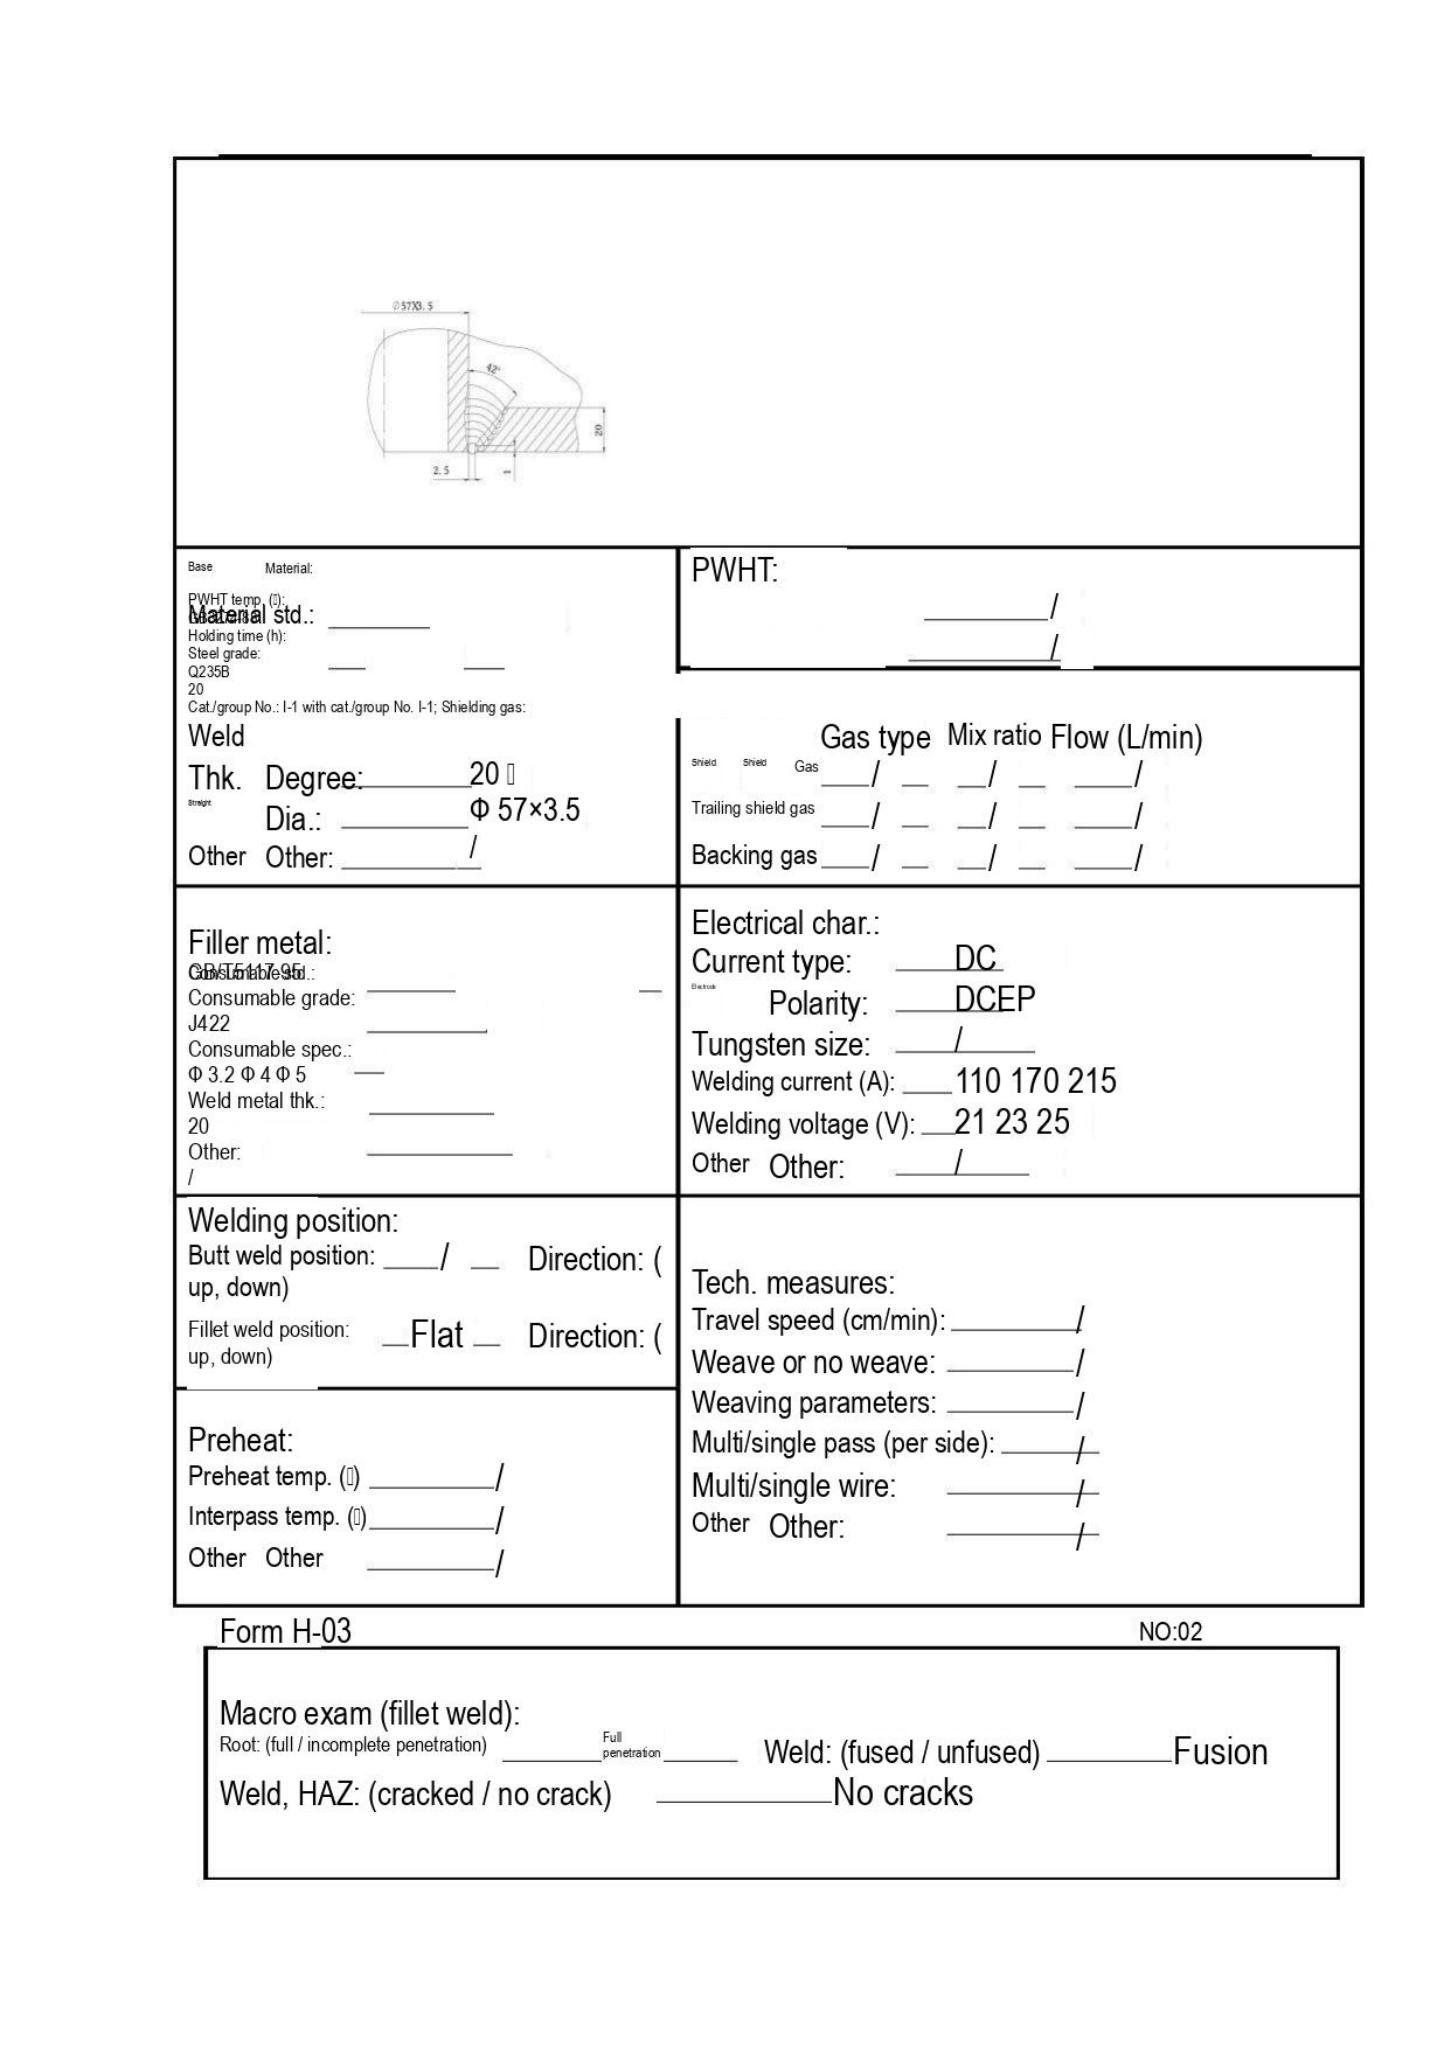Φ57X3.5

42°

20

2.5

1

Base Material:

PWHT temp. ():

Material std.:

Holding time (h):

Steel grade:

Q235B

20

Cat./group No.: I-1 with cat./group No. I-1; Shielding gas:

PWHT:

/

/

Weld

Thk. Degree: 20

Straight Dia.: Φ 57×3.5

Other Other: /

| | Gas type | Mix ratio | Flow (L/min) |
|---|---|---|---|
| Shield Shield Gas | / | / | / |
| Trailing shield gas | / | / | / |
| Backing gas | / | / | / |

Filler metal:

Consumable std.:

GB/T5117-95

Consumable grade:

J422

Consumable spec.:

Φ 3.2 Φ 4 Φ 5

Weld metal thk.:

20

Other:

/

Electrical char.:

Current type: DC

Electrode Polarity: DCEP

Tungsten size: /

Welding current (A): 110 170 215

Welding voltage (V): 21 23 25

Other Other: /

Welding position:

Butt weld position: / Direction: ( up, down)

Fillet weld position: Flat Direction: ( up, down)

Tech. measures:

Travel speed (cm/min): /

Weave or no weave: /

Weaving parameters: /

Multi/single pass (per side): /

Multi/single wire: /

Other Other: /

Preheat:

Preheat temp. () /

Interpass temp. () /

Other Other /

Form H-03

NO:02

Macro exam (fillet weld):

Root: (full / incomplete penetration) Full penetration

Weld: (fused / unfused) Fusion

Weld, HAZ: (cracked / no crack) No cracks
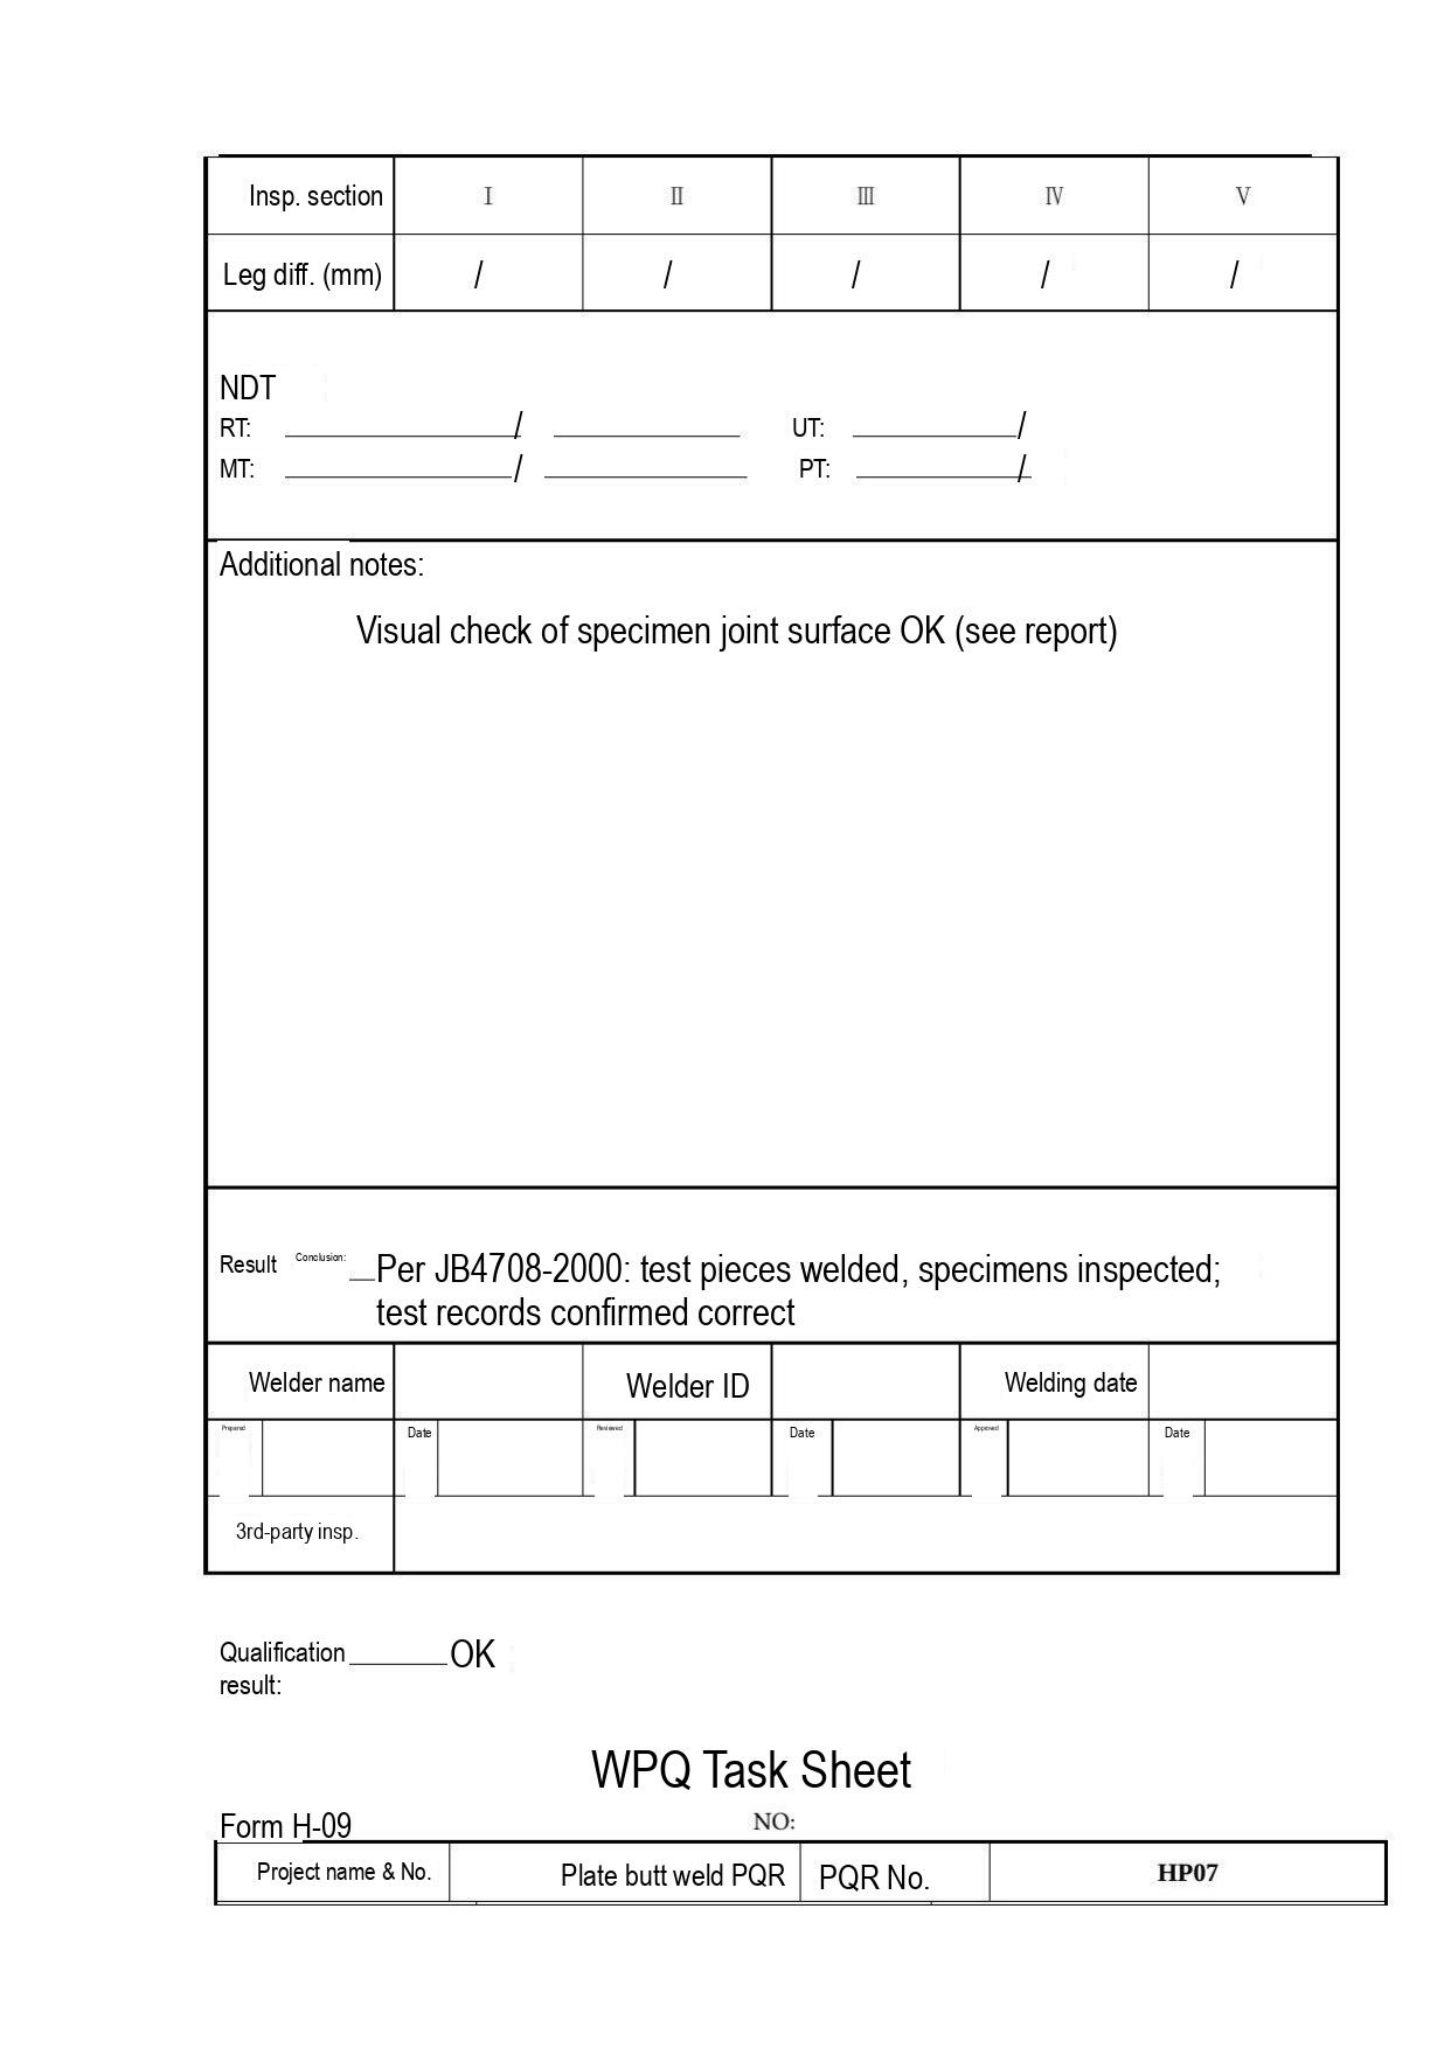| Insp. section | I | II | III | IV | V |
|---|---|---|---|---|---|
| Leg diff. (mm) | / | / | / | / | / |

NDT
RT: / UT: /
MT: / PT: /

Additional notes:

Visual check of specimen joint surface OK (see report)

Result Conclusion: Per JB4708-2000: test pieces welded, specimens inspected; test records confirmed correct

| Welder name | | Welder ID | | Welding date | |
|---|---|---|---|---|---|
| Prepared | Date | Reviewed | Date | Approved | Date |
| 3rd-party insp. | | | | | |

Qualification result: OK

WPQ Task Sheet

Form H-09 NO:

| Project name & No. | Plate butt weld PQR | PQR No. | HP07 |
|---|---|---|---|
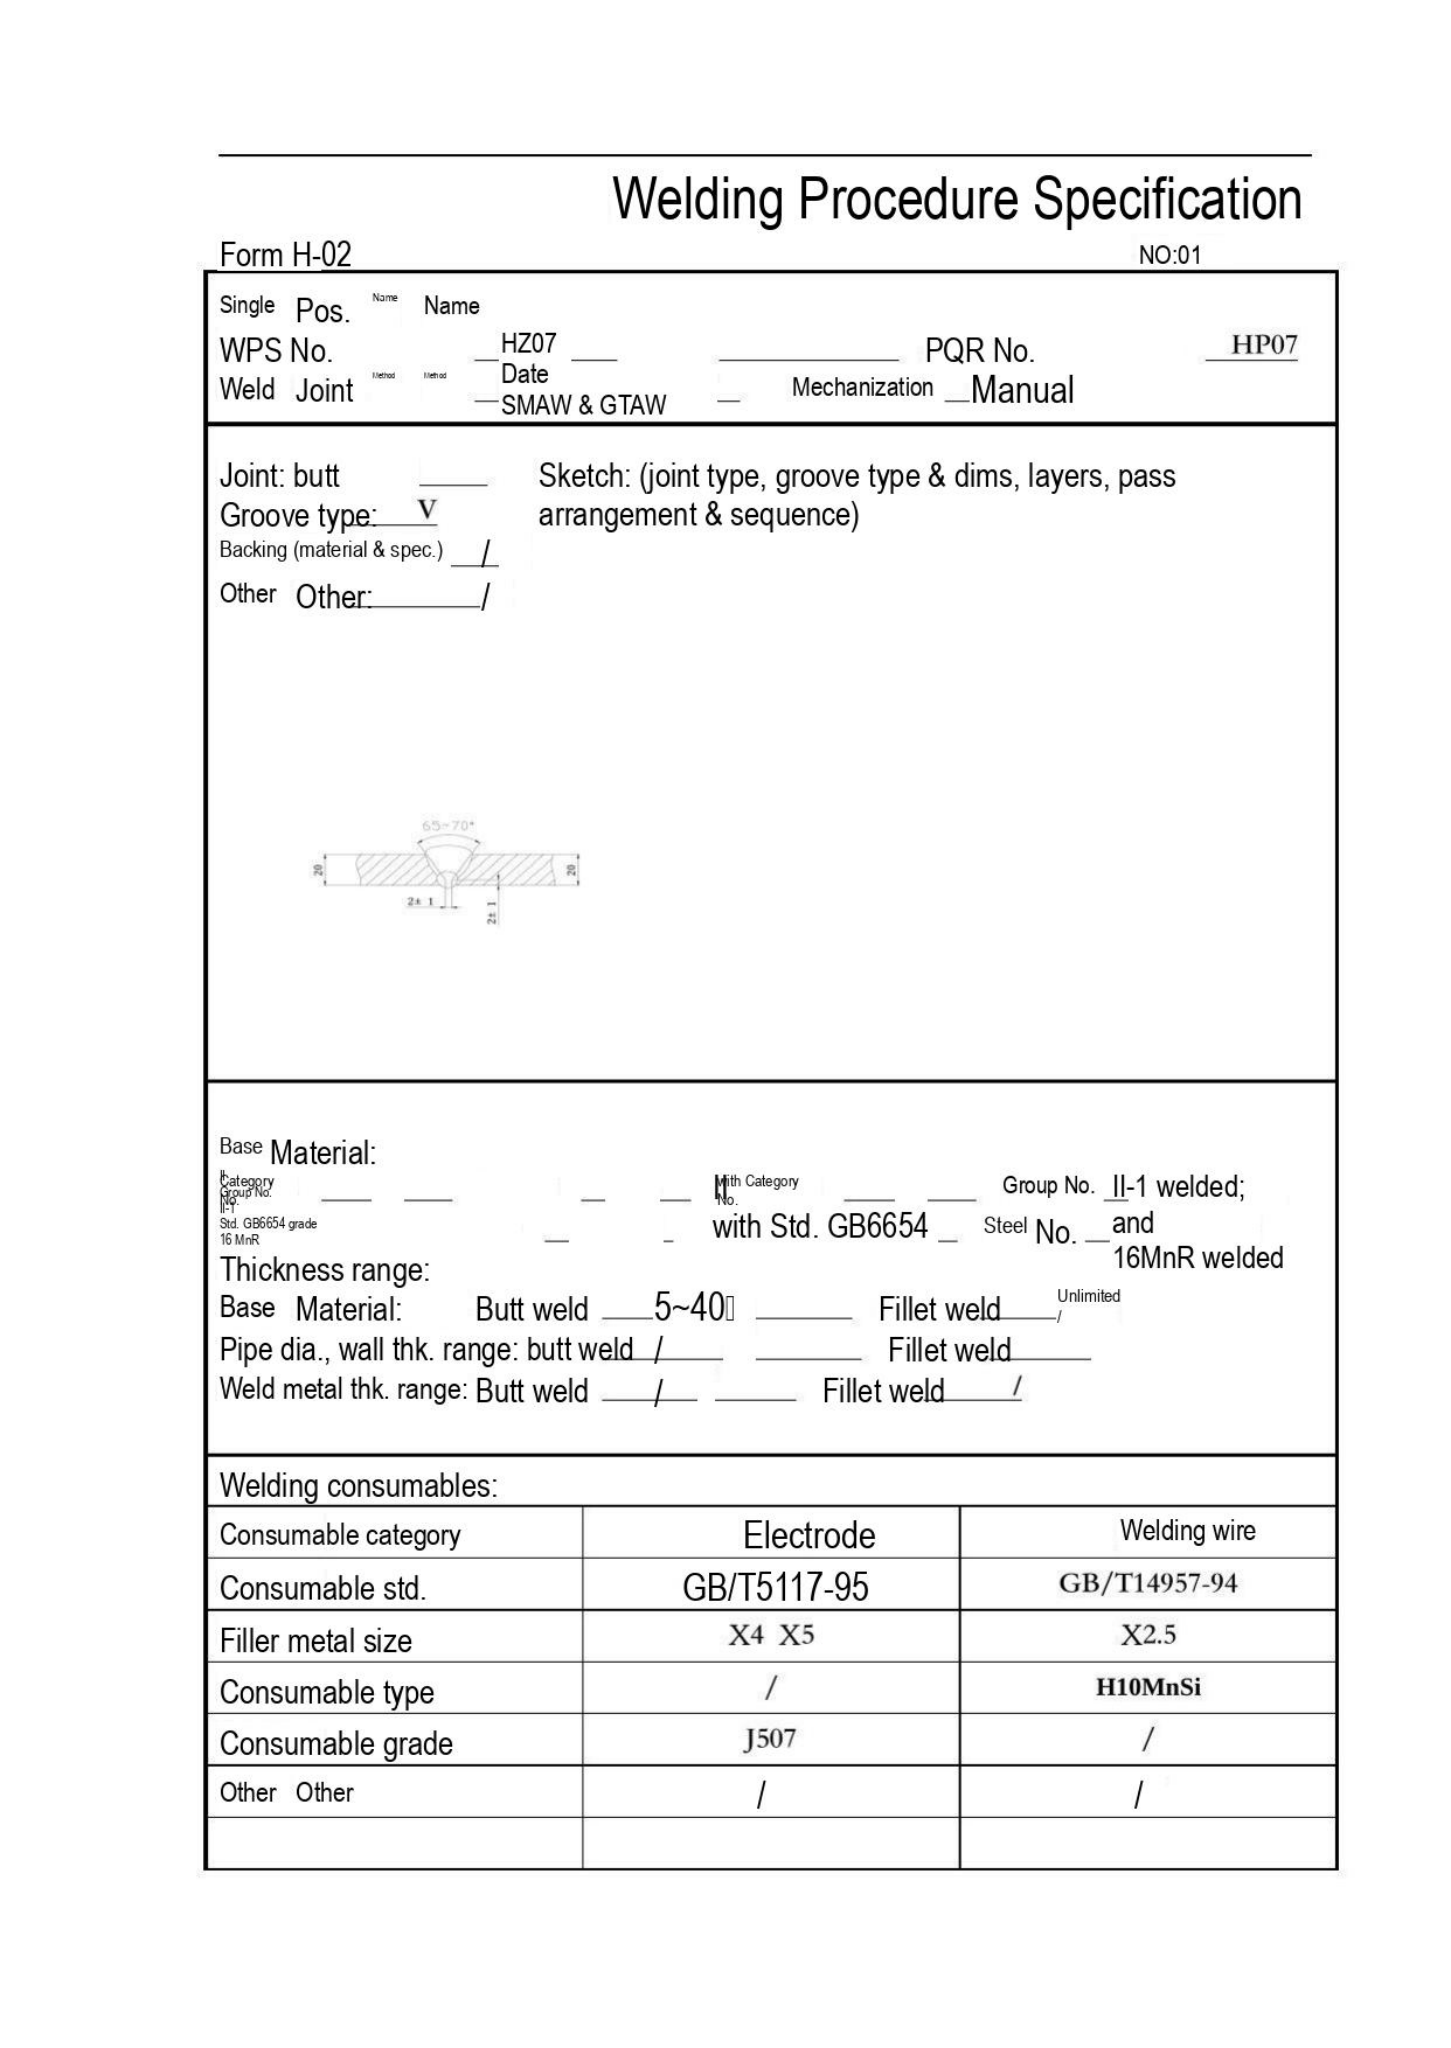Welding Procedure Specification

Form H-02 NO:01

Single Pos. Name Name
WPS No. HZ07 PQR No. HP07
Weld Joint Method Method Date SMAW & GTAW Mechanization Manual

Joint: butt
Groove type: V
Backing (material & spec.) /
Other Other: /

Sketch: (joint type, groove type & dims, layers, pass arrangement & sequence)

65~70°
20
20
2± 1
2± 1

Base Material:
II Category Group No. II-1
Std. GB6654 grade 16 MnR
II with Category No.
Group No. II-1 welded;
with Std. GB6654 Steel No. and 16MnR welded
Thickness range:
Base Material: Butt weld 5~40 Fillet weld Unlimited /
Pipe dia., wall thk. range: butt weld / Fillet weld
Weld metal thk. range: Butt weld / Fillet weld /

Welding consumables:

| Consumable category | Electrode | Welding wire |
|---|---|---|
| Consumable std. | GB/T5117-95 | GB/T14957-94 |
| Filler metal size | X4 X5 | X2.5 |
| Consumable type | / | H10MnSi |
| Consumable grade | J507 | / |
| Other Other | / | / |
| | | |
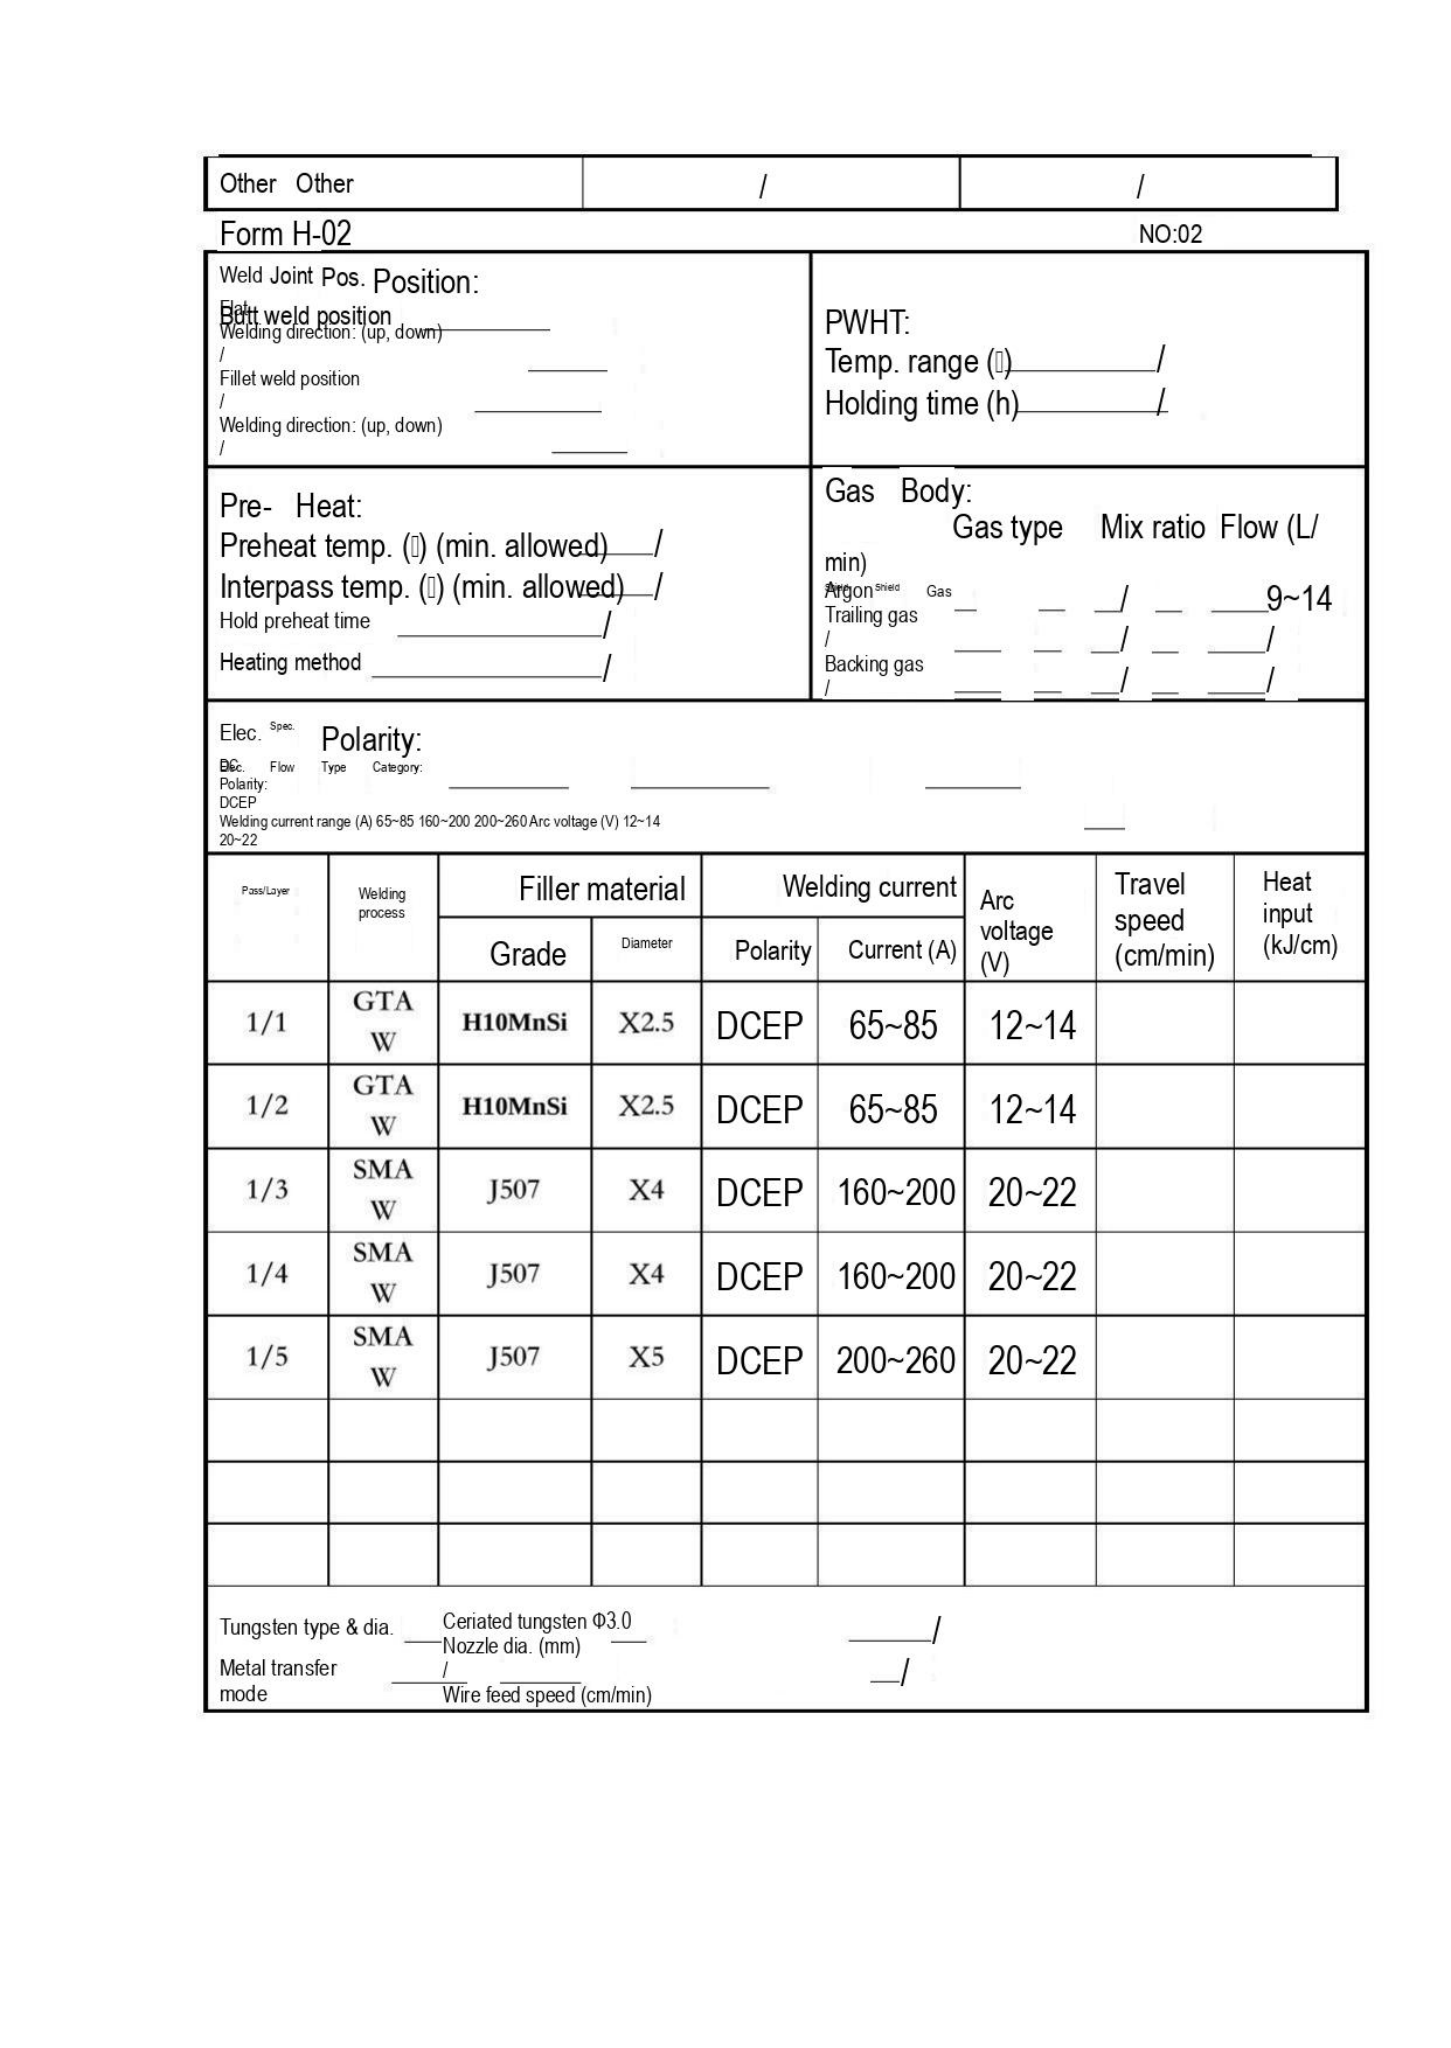| Other Other | / | / |
|---|---|---|

Form H-02

NO:02

Weld Joint Pos. Position:
Flat
Butt weld position
Welding direction: (up, down)
/
Fillet weld position
/
Welding direction: (up, down)
/

PWHT:
Temp. range (℃) /
Holding time (h) /

Pre- Heat:
Preheat temp. (℃) (min. allowed) /
Interpass temp. (℃) (min. allowed) /
Hold preheat time /
Heating method /

Gas Body:
Gas type Mix ratio Flow (L/min)
Shield Gas Argon / 9~14
Trailing gas / / /
Backing gas / / /

Elec. Spec. Polarity:
Elec. Flow Type Category: DC
Polarity:
DCEP
Welding current range (A) 65~85 160~200 200~260 Arc voltage (V) 12~14 20~22

| Pass/Layer | Welding process | Filler material: Grade | Filler material: Diameter | Welding current: Polarity | Welding current: Current (A) | Arc voltage (V) | Travel speed (cm/min) | Heat input (kJ/cm) |
|---|---|---|---|---|---|---|---|---|
| 1/1 | GTAW | H10MnSi | X2.5 | DCEP | 65~85 | 12~14 | | |
| 1/2 | GTAW | H10MnSi | X2.5 | DCEP | 65~85 | 12~14 | | |
| 1/3 | SMAW | J507 | X4 | DCEP | 160~200 | 20~22 | | |
| 1/4 | SMAW | J507 | X4 | DCEP | 160~200 | 20~22 | | |
| 1/5 | SMAW | J507 | X5 | DCEP | 200~260 | 20~22 | | |
| | | | | | | | | |
| | | | | | | | | |
| | | | | | | | | |

Tungsten type & dia. Ceriated tungsten Φ3.0
Nozzle dia. (mm) /
Metal transfer mode /
Wire feed speed (cm/min) /
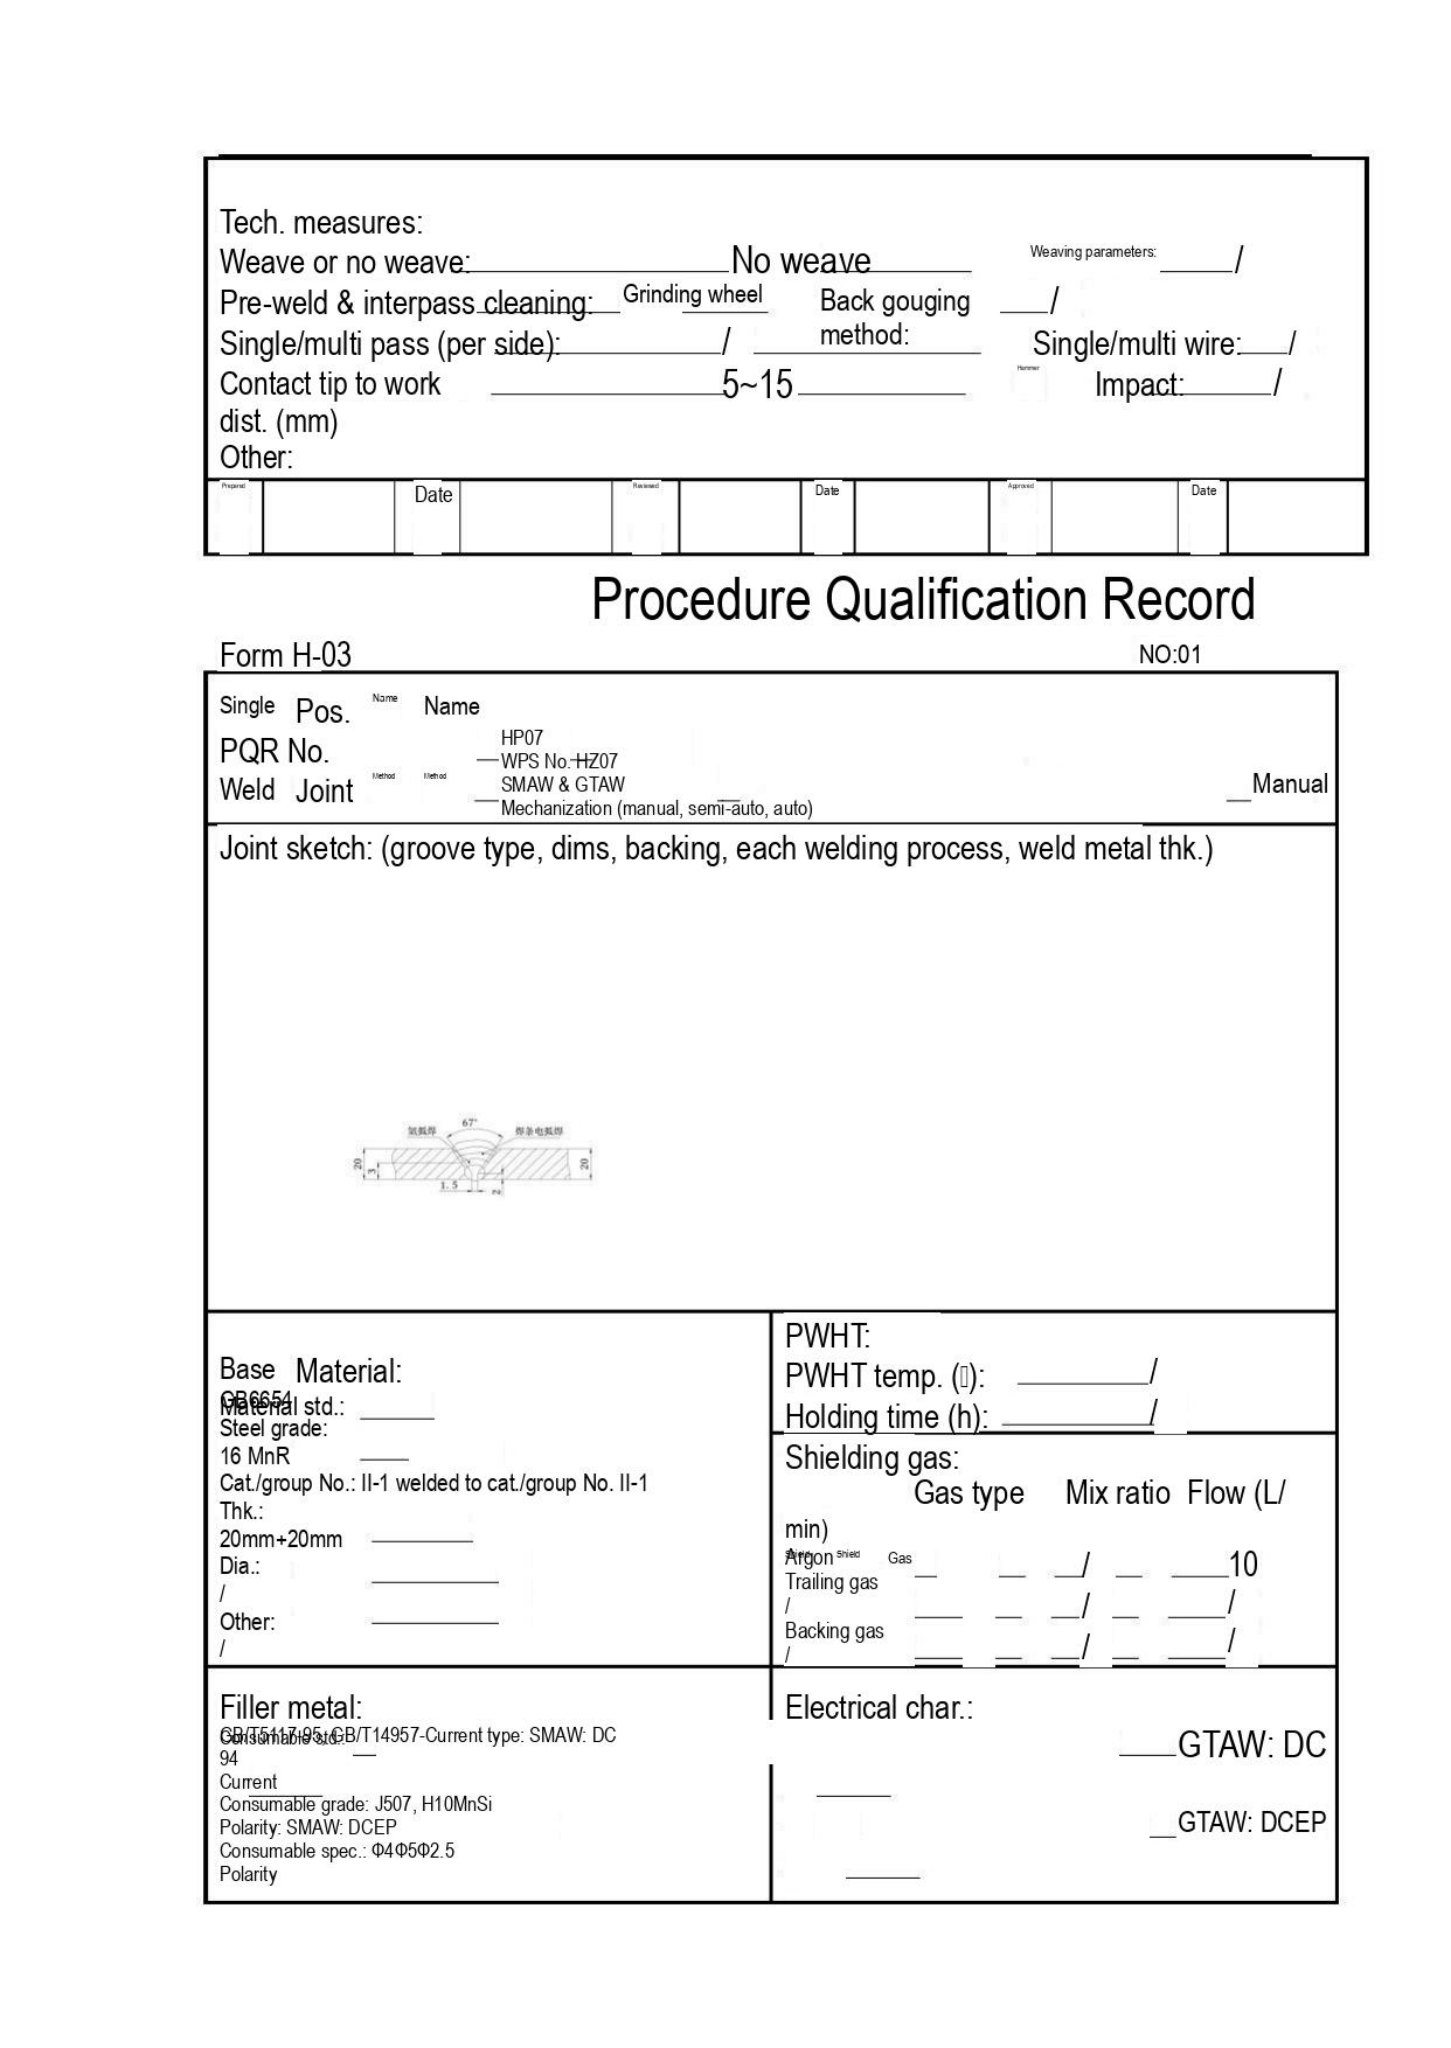Tech. measures:
Weave or no weave: No weave
Weaving parameters: /
Pre-weld & interpass cleaning: Grinding wheel
Back gouging method: /
Single/multi pass (per side): /
Single/multi wire: /
Contact tip to work dist. (mm) 5~15
Hammer
Impact: /
Other:

| Prepared | | Date | | Reviewed | | Date | | Approved | | Date | |
|---|---|---|---|---|---|---|---|---|---|---|---|

Procedure Qualification Record

Form H-03
NO:01

Single Pos. Name Name
PQR No. HP07
WPS No. HZ07
Weld Joint Method Method SMAW & GTAW
Mechanization (manual, semi-auto, auto) Manual

Joint sketch: (groove type, dims, backing, each welding process, weld metal thk.)

氩弧焊 67° 焊条电弧焊
20 3 20
1.5 P4

Base Material:
Material std.: GB6654
Steel grade: 16 MnR
Cat./group No.: II-1 welded to cat./group No. II-1
Thk.: 20mm+20mm
Dia.: /
Other: /

PWHT:
PWHT temp. (): /
Holding time (h): /

Shielding gas:
Gas type Mix ratio Flow (L/min)
Shield Gas Argon / 10
Trailing gas / /
Backing gas / /

Filler metal:
Consumable std.: GB/T5117-95, GB/T14957-94
Current type: SMAW: DC
Current
Consumable grade: J507, H10MnSi
Polarity: SMAW: DCEP
Consumable spec.: Φ4Φ5Φ2.5
Polarity

Electrical char.:
GTAW: DC
GTAW: DCEP
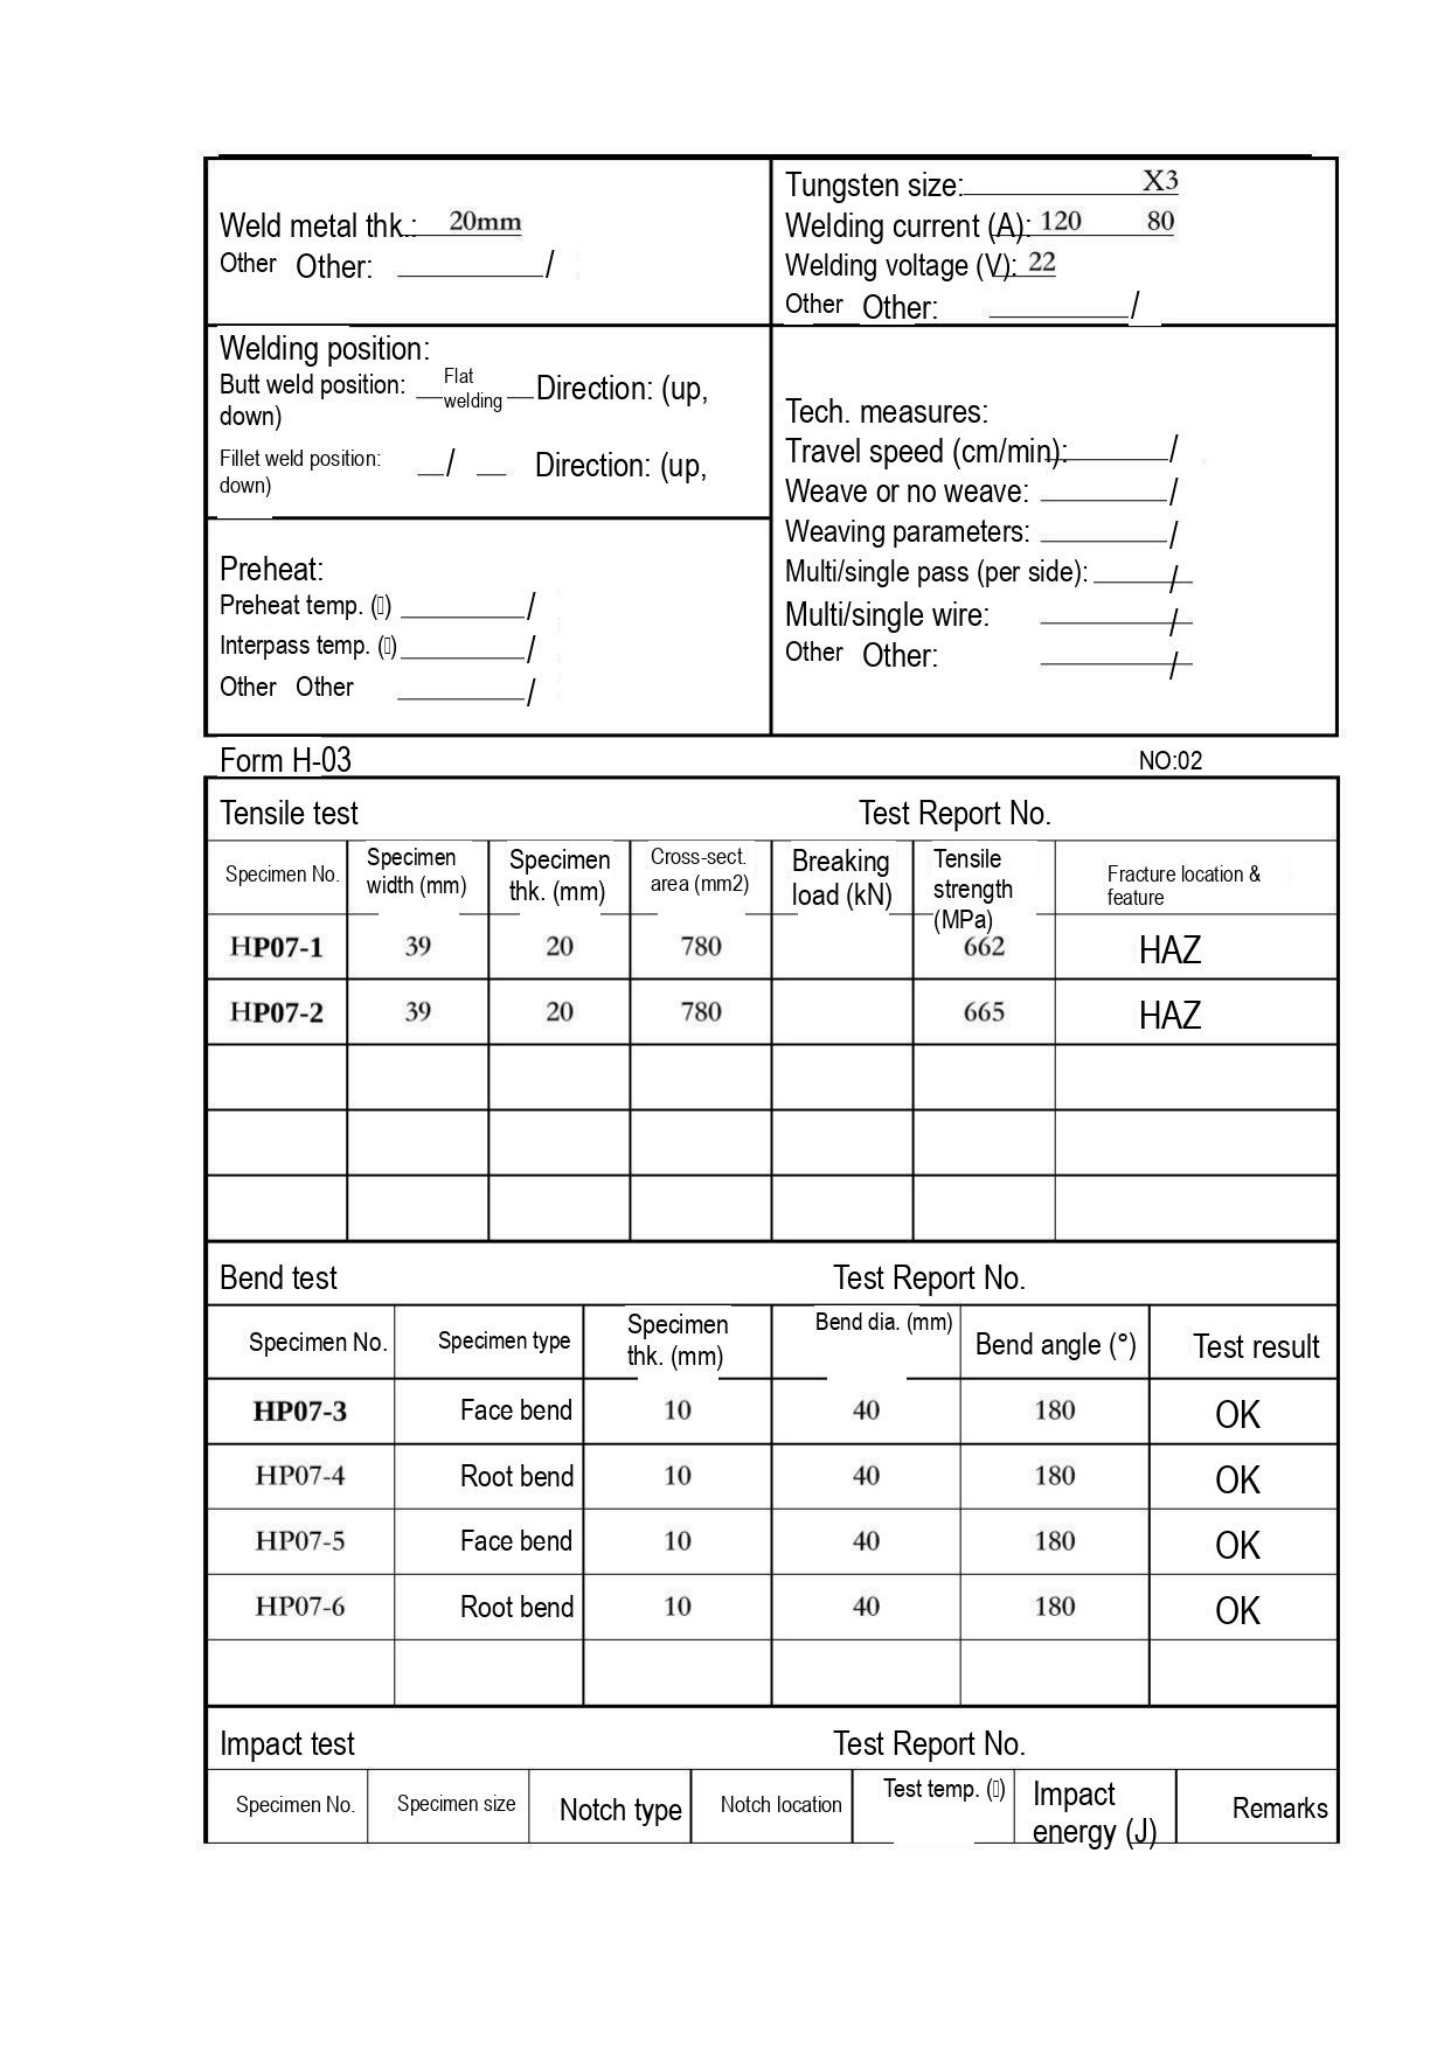| Weld metal thk.: 20mm<br>Other Other: / | Tungsten size: X3<br>Welding current (A): 120 80<br>Welding voltage (V): 22<br>Other Other: / |
|---|---|
| Welding position:<br>Butt weld position: Flat welding Direction: (up, down)<br>Fillet weld position: / Direction: (up, down) | Tech. measures:<br>Travel speed (cm/min): /<br>Weave or no weave: /<br>Weaving parameters: /<br>Multi/single pass (per side): /<br>Multi/single wire: /<br>Other Other: / |
| Preheat:<br>Preheat temp. ( ) /<br>Interpass temp. ( ) /<br>Other Other / | |

Form H-03 NO:02

Tensile test Test Report No.

| Specimen No. | Specimen width (mm) | Specimen thk. (mm) | Cross-sect. area (mm2) | Breaking load (kN) | Tensile strength (MPa) | Fracture location & feature |
|---|---|---|---|---|---|---|
| HP07-1 | 39 | 20 | 780 | | 662 | HAZ |
| HP07-2 | 39 | 20 | 780 | | 665 | HAZ |
| | | | | | | |
| | | | | | | |
| | | | | | | |

Bend test Test Report No.

| Specimen No. | Specimen type | Specimen thk. (mm) | Bend dia. (mm) | Bend angle (°) | Test result |
|---|---|---|---|---|---|
| HP07-3 | Face bend | 10 | 40 | 180 | OK |
| HP07-4 | Root bend | 10 | 40 | 180 | OK |
| HP07-5 | Face bend | 10 | 40 | 180 | OK |
| HP07-6 | Root bend | 10 | 40 | 180 | OK |
| | | | | | |

Impact test Test Report No.

| Specimen No. | Specimen size | Notch type | Notch location | Test temp. ( ) | Impact energy (J) | Remarks |
|---|---|---|---|---|---|---|
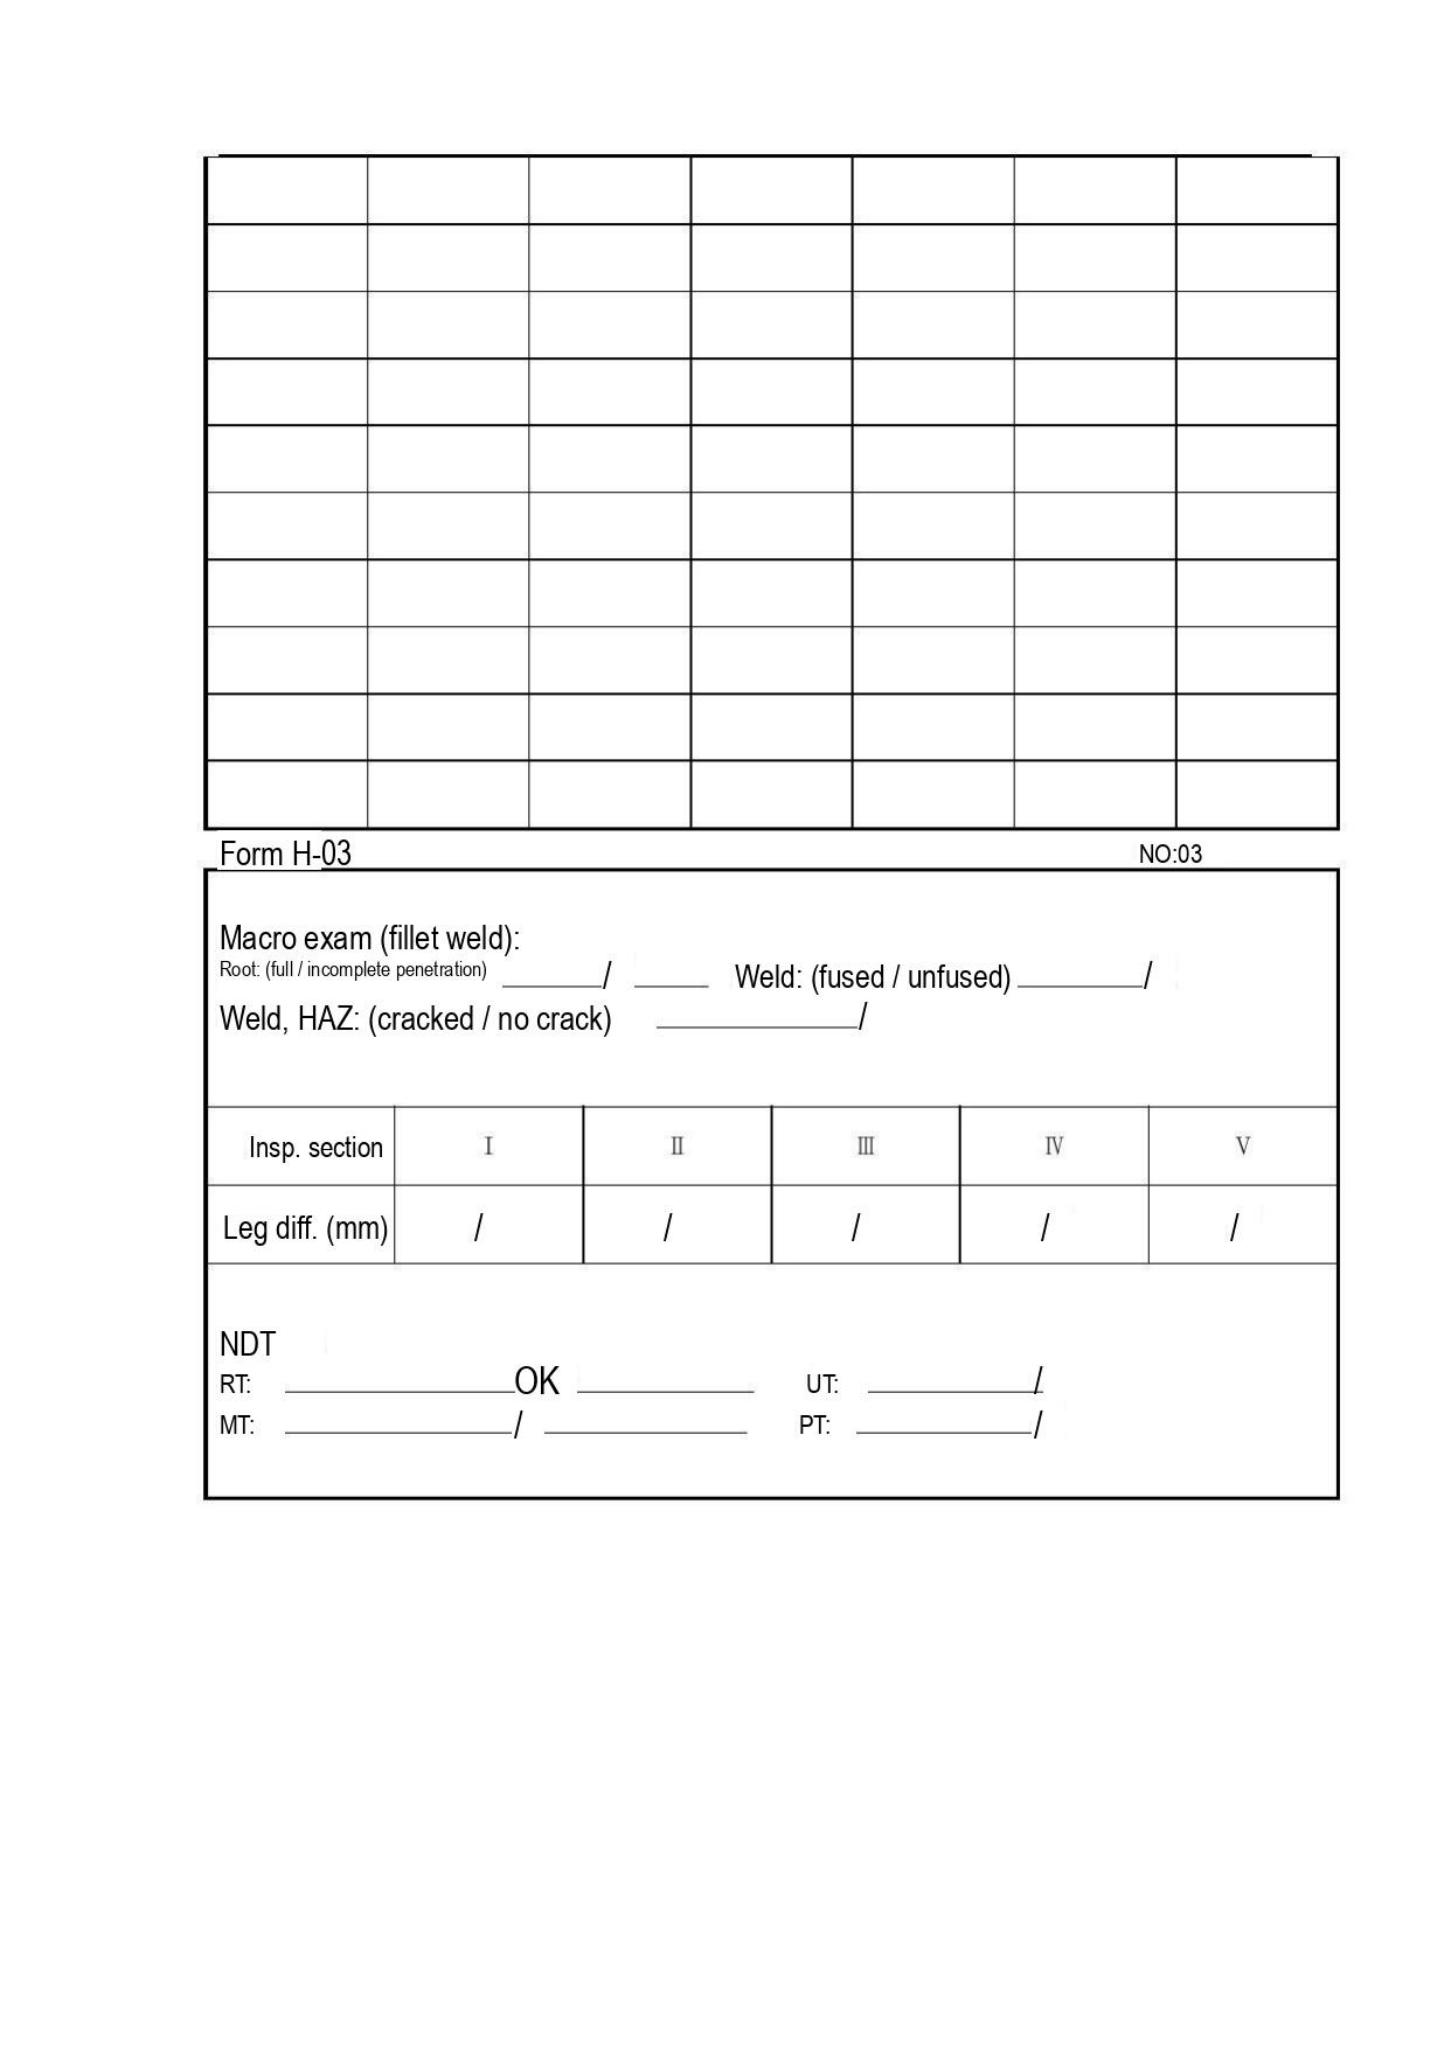|   |   |   |   |   |   |   |
|---|---|---|---|---|---|---|
|   |   |   |   |   |   |   |
|   |   |   |   |   |   |   |
|   |   |   |   |   |   |   |
|   |   |   |   |   |   |   |
|   |   |   |   |   |   |   |
|   |   |   |   |   |   |   |
|   |   |   |   |   |   |   |
|   |   |   |   |   |   |   |
|   |   |   |   |   |   |   |

Form H-03 NO:03

Macro exam (fillet weld):
Root: (full / incomplete penetration) ________/ _____ Weld: (fused / unfused) _________/
Weld, HAZ: (cracked / no crack) ______________/

| Insp. section | I | II | III | IV | V |
|---|---|---|---|---|---|
| Leg diff. (mm) | / | / | / | / | / |

NDT
RT: ______________OK ____________ UT: ____________/
MT: ______________/ ____________ PT: ____________/